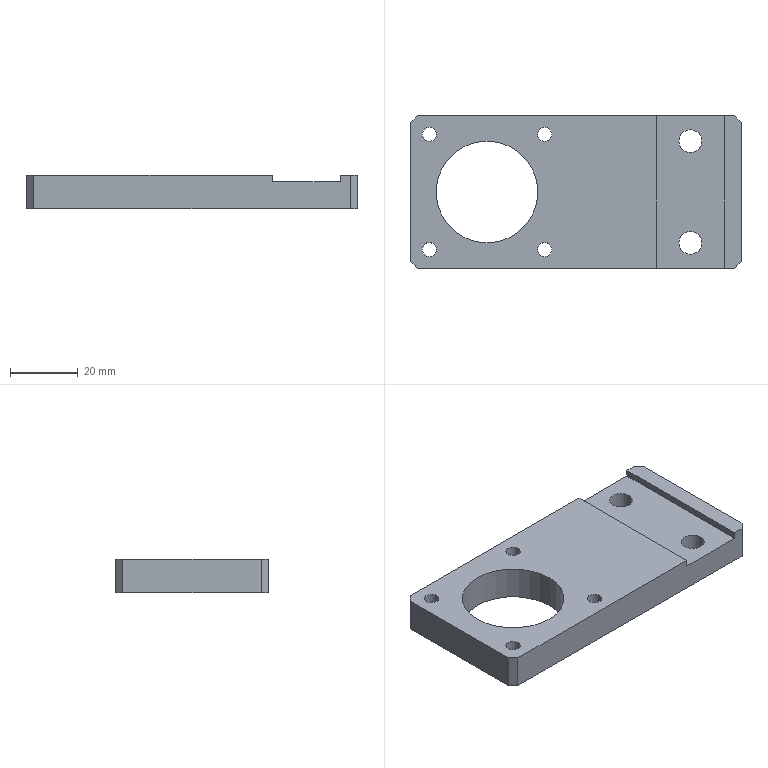Part | SolidWorks | features Chamfer 1, Extrusion 1, HoleWzd 1, ICE 1 | 1 solid | 28 faces | box 97.5 x 45 x 10 mm | volume 33791 mm3 | cylinder 14 | plane 14 | commonest cylinder face diameters 4.2 x8 6.8 x4 30 x2
STEP:
#1=CARTESIAN_POINT('',(41.6,5.5,10.));
#2=VERTEX_POINT('',#1);
#3=CARTESIAN_POINT('',(37.4,5.5,10.));
#4=VERTEX_POINT('',#3);
#5=CARTESIAN_POINT('',(39.5,5.5,10.));
#6=DIRECTION('',(0.,0.,-1.));
#7=DIRECTION('',(-1.,0.,0.));
#8=AXIS2_PLACEMENT_3D('',#5,#6,#7);
#9=CIRCLE('',#8,2.1);
#10=EDGE_CURVE('',#2,#4,#9,.T.);
#11=ORIENTED_EDGE('',*,*,#10,.F.);
#12=CARTESIAN_POINT('',(41.6,5.5,0.));
#13=VERTEX_POINT('',#12);
#14=CARTESIAN_POINT('',(41.6,5.5,0.));
#15=DIRECTION('',(0.,0.,-1.));
#16=VECTOR('',#15,1000.);
#17=LINE('',#14,#16);
#18=EDGE_CURVE('',#2,#13,#17,.T.);
#19=ORIENTED_EDGE('',*,*,#18,.T.);
#20=CARTESIAN_POINT('',(37.4,5.5,0.));
#21=VERTEX_POINT('',#20);
#22=CARTESIAN_POINT('',(39.5,5.5,0.));
#23=DIRECTION('',(0.,0.,-1.));
#24=DIRECTION('',(-1.,0.,0.));
#25=AXIS2_PLACEMENT_3D('',#22,#23,#24);
#26=CIRCLE('',#25,2.1);
#27=EDGE_CURVE('',#13,#21,#26,.T.);
#28=ORIENTED_EDGE('',*,*,#27,.T.);
#29=CARTESIAN_POINT('',(37.4,5.5,0.));
#30=DIRECTION('',(0.,0.,-1.));
#31=VECTOR('',#30,1000.);
#32=LINE('',#29,#31);
#33=EDGE_CURVE('',#4,#21,#32,.T.);
#34=ORIENTED_EDGE('',*,*,#33,.F.);
#35=EDGE_LOOP('',(#11,#19,#28,#34));
#36=FACE_OUTER_BOUND('',#35,.T.);
#37=CARTESIAN_POINT('',(39.5,5.5,0.));
#38=DIRECTION('',(0.,0.,-1.));
#39=DIRECTION('',(-1.,0.,0.));
#40=AXIS2_PLACEMENT_3D('',#37,#38,#39);
#41=CYLINDRICAL_SURFACE('',#40,2.1);
#42=ADVANCED_FACE('',(#36),#41,.F.);
#43=CARTESIAN_POINT('',(7.6,5.5,10.));
#44=VERTEX_POINT('',#43);
#45=CARTESIAN_POINT('',(3.4,5.5,10.));
#46=VERTEX_POINT('',#45);
#47=CARTESIAN_POINT('',(5.5,5.5,10.));
#48=DIRECTION('',(0.,0.,-1.));
#49=DIRECTION('',(-1.,0.,0.));
#50=AXIS2_PLACEMENT_3D('',#47,#48,#49);
#51=CIRCLE('',#50,2.1);
#52=EDGE_CURVE('',#44,#46,#51,.T.);
#53=ORIENTED_EDGE('',*,*,#52,.F.);
#54=CARTESIAN_POINT('',(7.6,5.5,0.));
#55=VERTEX_POINT('',#54);
#56=CARTESIAN_POINT('',(7.6,5.5,0.));
#57=DIRECTION('',(0.,0.,-1.));
#58=VECTOR('',#57,1000.);
#59=LINE('',#56,#58);
#60=EDGE_CURVE('',#44,#55,#59,.T.);
#61=ORIENTED_EDGE('',*,*,#60,.T.);
#62=CARTESIAN_POINT('',(3.4,5.5,0.));
#63=VERTEX_POINT('',#62);
#64=CARTESIAN_POINT('',(5.5,5.5,0.));
#65=DIRECTION('',(0.,0.,-1.));
#66=DIRECTION('',(-1.,0.,0.));
#67=AXIS2_PLACEMENT_3D('',#64,#65,#66);
#68=CIRCLE('',#67,2.1);
#69=EDGE_CURVE('',#55,#63,#68,.T.);
#70=ORIENTED_EDGE('',*,*,#69,.T.);
#71=CARTESIAN_POINT('',(3.4,5.5,0.));
#72=DIRECTION('',(0.,0.,-1.));
#73=VECTOR('',#72,1000.);
#74=LINE('',#71,#73);
#75=EDGE_CURVE('',#46,#63,#74,.T.);
#76=ORIENTED_EDGE('',*,*,#75,.F.);
#77=EDGE_LOOP('',(#53,#61,#70,#76));
#78=FACE_OUTER_BOUND('',#77,.T.);
#79=CARTESIAN_POINT('',(5.5,5.5,0.));
#80=DIRECTION('',(0.,0.,-1.));
#81=DIRECTION('',(-1.,0.,0.));
#82=AXIS2_PLACEMENT_3D('',#79,#80,#81);
#83=CYLINDRICAL_SURFACE('',#82,2.1);
#84=ADVANCED_FACE('',(#78),#83,.F.);
#85=CARTESIAN_POINT('',(7.6,39.5,10.));
#86=VERTEX_POINT('',#85);
#87=CARTESIAN_POINT('',(3.4,39.5,10.));
#88=VERTEX_POINT('',#87);
#89=CARTESIAN_POINT('',(5.5,39.5,10.));
#90=DIRECTION('',(0.,0.,-1.));
#91=DIRECTION('',(-1.,0.,0.));
#92=AXIS2_PLACEMENT_3D('',#89,#90,#91);
#93=CIRCLE('',#92,2.1);
#94=EDGE_CURVE('',#86,#88,#93,.T.);
#95=ORIENTED_EDGE('',*,*,#94,.F.);
#96=CARTESIAN_POINT('',(7.6,39.5,0.));
#97=VERTEX_POINT('',#96);
#98=CARTESIAN_POINT('',(7.6,39.5,0.));
#99=DIRECTION('',(0.,0.,-1.));
#100=VECTOR('',#99,1000.);
#101=LINE('',#98,#100);
#102=EDGE_CURVE('',#86,#97,#101,.T.);
#103=ORIENTED_EDGE('',*,*,#102,.T.);
#104=CARTESIAN_POINT('',(3.4,39.5,0.));
#105=VERTEX_POINT('',#104);
#106=CARTESIAN_POINT('',(5.5,39.5,0.));
#107=DIRECTION('',(0.,0.,-1.));
#108=DIRECTION('',(-1.,0.,0.));
#109=AXIS2_PLACEMENT_3D('',#106,#107,#108);
#110=CIRCLE('',#109,2.1);
#111=EDGE_CURVE('',#97,#105,#110,.T.);
#112=ORIENTED_EDGE('',*,*,#111,.T.);
#113=CARTESIAN_POINT('',(3.4,39.5,0.));
#114=DIRECTION('',(0.,0.,-1.));
#115=VECTOR('',#114,1000.);
#116=LINE('',#113,#115);
#117=EDGE_CURVE('',#88,#105,#116,.T.);
#118=ORIENTED_EDGE('',*,*,#117,.F.);
#119=EDGE_LOOP('',(#95,#103,#112,#118));
#120=FACE_OUTER_BOUND('',#119,.T.);
#121=CARTESIAN_POINT('',(5.5,39.5,0.));
#122=DIRECTION('',(0.,0.,-1.));
#123=DIRECTION('',(-1.,0.,0.));
#124=AXIS2_PLACEMENT_3D('',#121,#122,#123);
#125=CYLINDRICAL_SURFACE('',#124,2.1);
#126=ADVANCED_FACE('',(#120),#125,.F.);
#127=CARTESIAN_POINT('',(41.6,39.5,10.));
#128=VERTEX_POINT('',#127);
#129=CARTESIAN_POINT('',(37.4,39.5,10.));
#130=VERTEX_POINT('',#129);
#131=CARTESIAN_POINT('',(39.5,39.5,10.));
#132=DIRECTION('',(0.,0.,-1.));
#133=DIRECTION('',(-1.,0.,0.));
#134=AXIS2_PLACEMENT_3D('',#131,#132,#133);
#135=CIRCLE('',#134,2.1);
#136=EDGE_CURVE('',#128,#130,#135,.T.);
#137=ORIENTED_EDGE('',*,*,#136,.F.);
#138=CARTESIAN_POINT('',(41.6,39.5,0.));
#139=VERTEX_POINT('',#138);
#140=CARTESIAN_POINT('',(41.6,39.5,0.));
#141=DIRECTION('',(0.,0.,-1.));
#142=VECTOR('',#141,1000.);
#143=LINE('',#140,#142);
#144=EDGE_CURVE('',#128,#139,#143,.T.);
#145=ORIENTED_EDGE('',*,*,#144,.T.);
#146=CARTESIAN_POINT('',(37.4,39.5,0.));
#147=VERTEX_POINT('',#146);
#148=CARTESIAN_POINT('',(39.5,39.5,0.));
#149=DIRECTION('',(0.,0.,-1.));
#150=DIRECTION('',(-1.,0.,0.));
#151=AXIS2_PLACEMENT_3D('',#148,#149,#150);
#152=CIRCLE('',#151,2.1);
#153=EDGE_CURVE('',#139,#147,#152,.T.);
#154=ORIENTED_EDGE('',*,*,#153,.T.);
#155=CARTESIAN_POINT('',(37.4,39.5,0.));
#156=DIRECTION('',(0.,0.,-1.));
#157=VECTOR('',#156,1000.);
#158=LINE('',#155,#157);
#159=EDGE_CURVE('',#130,#147,#158,.T.);
#160=ORIENTED_EDGE('',*,*,#159,.F.);
#161=EDGE_LOOP('',(#137,#145,#154,#160));
#162=FACE_OUTER_BOUND('',#161,.T.);
#163=CARTESIAN_POINT('',(39.5,39.5,0.));
#164=DIRECTION('',(0.,0.,-1.));
#165=DIRECTION('',(-1.,0.,0.));
#166=AXIS2_PLACEMENT_3D('',#163,#164,#165);
#167=CYLINDRICAL_SURFACE('',#166,2.1);
#168=ADVANCED_FACE('',(#162),#167,.F.);
#169=CARTESIAN_POINT('',(79.1,7.5,8.));
#170=VERTEX_POINT('',#169);
#171=CARTESIAN_POINT('',(85.9,7.5,8.));
#172=VERTEX_POINT('',#171);
#173=CARTESIAN_POINT('',(82.5,7.5,8.));
#174=DIRECTION('',(0.,0.,1.));
#175=DIRECTION('',(-1.,0.,0.));
#176=AXIS2_PLACEMENT_3D('',#173,#174,#175);
#177=CIRCLE('',#176,3.4);
#178=EDGE_CURVE('',#170,#172,#177,.T.);
#179=ORIENTED_EDGE('',*,*,#178,.T.);
#180=CARTESIAN_POINT('',(85.9,7.5,0.));
#181=VERTEX_POINT('',#180);
#182=CARTESIAN_POINT('',(85.9,7.5,10.));
#183=DIRECTION('',(0.,0.,-1.));
#184=VECTOR('',#183,1000.);
#185=LINE('',#182,#184);
#186=EDGE_CURVE('',#172,#181,#185,.T.);
#187=ORIENTED_EDGE('',*,*,#186,.T.);
#188=CARTESIAN_POINT('',(79.1,7.5,0.));
#189=VERTEX_POINT('',#188);
#190=CARTESIAN_POINT('',(82.5,7.5,0.));
#191=DIRECTION('',(0.,0.,1.));
#192=DIRECTION('',(1.,0.,0.));
#193=AXIS2_PLACEMENT_3D('',#190,#191,#192);
#194=CIRCLE('',#193,3.4);
#195=EDGE_CURVE('',#189,#181,#194,.T.);
#196=ORIENTED_EDGE('',*,*,#195,.F.);
#197=CARTESIAN_POINT('',(79.1,7.5,10.));
#198=DIRECTION('',(0.,0.,-1.));
#199=VECTOR('',#198,1000.);
#200=LINE('',#197,#199);
#201=EDGE_CURVE('',#170,#189,#200,.T.);
#202=ORIENTED_EDGE('',*,*,#201,.F.);
#203=EDGE_LOOP('',(#179,#187,#196,#202));
#204=FACE_OUTER_BOUND('',#203,.T.);
#205=CARTESIAN_POINT('',(82.5,7.5,10.));
#206=DIRECTION('',(0.,0.,-1.));
#207=DIRECTION('',(-1.,0.,0.));
#208=AXIS2_PLACEMENT_3D('',#205,#206,#207);
#209=CYLINDRICAL_SURFACE('',#208,3.4);
#210=ADVANCED_FACE('',(#204),#209,.F.);
#211=CARTESIAN_POINT('',(79.1,37.5,8.));
#212=VERTEX_POINT('',#211);
#213=CARTESIAN_POINT('',(85.9,37.5,8.));
#214=VERTEX_POINT('',#213);
#215=CARTESIAN_POINT('',(82.5,37.5,8.));
#216=DIRECTION('',(0.,0.,1.));
#217=DIRECTION('',(-1.,0.,0.));
#218=AXIS2_PLACEMENT_3D('',#215,#216,#217);
#219=CIRCLE('',#218,3.4);
#220=EDGE_CURVE('',#212,#214,#219,.T.);
#221=ORIENTED_EDGE('',*,*,#220,.T.);
#222=CARTESIAN_POINT('',(85.9,37.5,0.));
#223=VERTEX_POINT('',#222);
#224=CARTESIAN_POINT('',(85.9,37.5,10.));
#225=DIRECTION('',(0.,0.,-1.));
#226=VECTOR('',#225,1000.);
#227=LINE('',#224,#226);
#228=EDGE_CURVE('',#214,#223,#227,.T.);
#229=ORIENTED_EDGE('',*,*,#228,.T.);
#230=CARTESIAN_POINT('',(79.1,37.5,0.));
#231=VERTEX_POINT('',#230);
#232=CARTESIAN_POINT('',(82.5,37.5,0.));
#233=DIRECTION('',(0.,0.,1.));
#234=DIRECTION('',(1.,0.,0.));
#235=AXIS2_PLACEMENT_3D('',#232,#233,#234);
#236=CIRCLE('',#235,3.4);
#237=EDGE_CURVE('',#231,#223,#236,.T.);
#238=ORIENTED_EDGE('',*,*,#237,.F.);
#239=CARTESIAN_POINT('',(79.1,37.5,10.));
#240=DIRECTION('',(0.,0.,-1.));
#241=VECTOR('',#240,1000.);
#242=LINE('',#239,#241);
#243=EDGE_CURVE('',#212,#231,#242,.T.);
#244=ORIENTED_EDGE('',*,*,#243,.F.);
#245=EDGE_LOOP('',(#221,#229,#238,#244));
#246=FACE_OUTER_BOUND('',#245,.T.);
#247=CARTESIAN_POINT('',(82.5,37.5,10.));
#248=DIRECTION('',(0.,0.,-1.));
#249=DIRECTION('',(-1.,0.,0.));
#250=AXIS2_PLACEMENT_3D('',#247,#248,#249);
#251=CYLINDRICAL_SURFACE('',#250,3.4);
#252=ADVANCED_FACE('',(#246),#251,.F.);
#253=CARTESIAN_POINT('',(7.5,22.5,10.));
#254=VERTEX_POINT('',#253);
#255=CARTESIAN_POINT('',(37.5,22.5,10.));
#256=VERTEX_POINT('',#255);
#257=CARTESIAN_POINT('',(22.5,22.5,10.));
#258=DIRECTION('',(0.,0.,1.));
#259=DIRECTION('',(1.,0.,0.));
#260=AXIS2_PLACEMENT_3D('',#257,#258,#259);
#261=CIRCLE('',#260,15.);
#262=EDGE_CURVE('',#254,#256,#261,.T.);
#263=ORIENTED_EDGE('',*,*,#262,.T.);
#264=CARTESIAN_POINT('',(37.5,22.5,0.));
#265=VERTEX_POINT('',#264);
#266=CARTESIAN_POINT('',(37.5,22.5,10.));
#267=DIRECTION('',(0.,0.,-1.));
#268=VECTOR('',#267,1000.);
#269=LINE('',#266,#268);
#270=EDGE_CURVE('',#256,#265,#269,.T.);
#271=ORIENTED_EDGE('',*,*,#270,.T.);
#272=CARTESIAN_POINT('',(7.5,22.5,0.));
#273=VERTEX_POINT('',#272);
#274=CARTESIAN_POINT('',(22.5,22.5,0.));
#275=DIRECTION('',(0.,0.,1.));
#276=DIRECTION('',(1.,0.,0.));
#277=AXIS2_PLACEMENT_3D('',#274,#275,#276);
#278=CIRCLE('',#277,15.);
#279=EDGE_CURVE('',#273,#265,#278,.T.);
#280=ORIENTED_EDGE('',*,*,#279,.F.);
#281=CARTESIAN_POINT('',(7.5,22.5,10.));
#282=DIRECTION('',(0.,0.,-1.));
#283=VECTOR('',#282,1000.);
#284=LINE('',#281,#283);
#285=EDGE_CURVE('',#254,#273,#284,.T.);
#286=ORIENTED_EDGE('',*,*,#285,.F.);
#287=EDGE_LOOP('',(#263,#271,#280,#286));
#288=FACE_OUTER_BOUND('',#287,.T.);
#289=CARTESIAN_POINT('',(22.5,22.5,10.));
#290=DIRECTION('',(0.,0.,-1.));
#291=DIRECTION('',(-1.,0.,0.));
#292=AXIS2_PLACEMENT_3D('',#289,#290,#291);
#293=CYLINDRICAL_SURFACE('',#292,15.);
#294=ADVANCED_FACE('',(#288),#293,.F.);
#295=CARTESIAN_POINT('',(39.5,5.5,10.));
#296=DIRECTION('',(0.,0.,-1.));
#297=DIRECTION('',(-1.,0.,0.));
#298=AXIS2_PLACEMENT_3D('',#295,#296,#297);
#299=CIRCLE('',#298,2.1);
#300=EDGE_CURVE('',#4,#2,#299,.T.);
#301=ORIENTED_EDGE('',*,*,#300,.T.);
#302=ORIENTED_EDGE('',*,*,#10,.T.);
#303=EDGE_LOOP('',(#301,#302));
#304=FACE_BOUND('',#303,.T.);
#305=CARTESIAN_POINT('',(5.5,5.5,10.));
#306=DIRECTION('',(0.,0.,-1.));
#307=DIRECTION('',(-1.,0.,0.));
#308=AXIS2_PLACEMENT_3D('',#305,#306,#307);
#309=CIRCLE('',#308,2.1);
#310=EDGE_CURVE('',#46,#44,#309,.T.);
#311=ORIENTED_EDGE('',*,*,#310,.T.);
#312=ORIENTED_EDGE('',*,*,#52,.T.);
#313=EDGE_LOOP('',(#311,#312));
#314=FACE_BOUND('',#313,.T.);
#315=CARTESIAN_POINT('',(5.5,39.5,10.));
#316=DIRECTION('',(0.,0.,-1.));
#317=DIRECTION('',(-1.,0.,0.));
#318=AXIS2_PLACEMENT_3D('',#315,#316,#317);
#319=CIRCLE('',#318,2.1);
#320=EDGE_CURVE('',#88,#86,#319,.T.);
#321=ORIENTED_EDGE('',*,*,#320,.T.);
#322=ORIENTED_EDGE('',*,*,#94,.T.);
#323=EDGE_LOOP('',(#321,#322));
#324=FACE_BOUND('',#323,.T.);
#325=CARTESIAN_POINT('',(39.5,39.5,10.));
#326=DIRECTION('',(0.,0.,-1.));
#327=DIRECTION('',(-1.,0.,0.));
#328=AXIS2_PLACEMENT_3D('',#325,#326,#327);
#329=CIRCLE('',#328,2.1);
#330=EDGE_CURVE('',#130,#128,#329,.T.);
#331=ORIENTED_EDGE('',*,*,#330,.T.);
#332=ORIENTED_EDGE('',*,*,#136,.T.);
#333=EDGE_LOOP('',(#331,#332));
#334=FACE_BOUND('',#333,.T.);
#335=ORIENTED_EDGE('',*,*,#262,.F.);
#336=CARTESIAN_POINT('',(22.5,22.5,10.));
#337=DIRECTION('',(0.,0.,1.));
#338=DIRECTION('',(1.,0.,0.));
#339=AXIS2_PLACEMENT_3D('',#336,#337,#338);
#340=CIRCLE('',#339,15.);
#341=EDGE_CURVE('',#256,#254,#340,.T.);
#342=ORIENTED_EDGE('',*,*,#341,.F.);
#343=EDGE_LOOP('',(#335,#342));
#344=FACE_BOUND('',#343,.T.);
#345=CARTESIAN_POINT('',(0.,43.,10.));
#346=VERTEX_POINT('',#345);
#347=CARTESIAN_POINT('',(0.,2.,10.));
#348=VERTEX_POINT('',#347);
#349=CARTESIAN_POINT('',(0.,0.,10.));
#350=DIRECTION('',(0.,-1.,0.));
#351=VECTOR('',#350,1000.);
#352=LINE('',#349,#351);
#353=EDGE_CURVE('',#346,#348,#352,.T.);
#354=ORIENTED_EDGE('',*,*,#353,.T.);
#355=CARTESIAN_POINT('',(2.,0.,10.));
#356=VERTEX_POINT('',#355);
#357=CARTESIAN_POINT('',(2.,0.,10.));
#358=DIRECTION('',(0.7071,-0.7071,0.));
#359=VECTOR('',#358,1000.);
#360=LINE('',#357,#359);
#361=EDGE_CURVE('',#348,#356,#360,.T.);
#362=ORIENTED_EDGE('',*,*,#361,.T.);
#363=CARTESIAN_POINT('',(72.5,0.,10.));
#364=VERTEX_POINT('',#363);
#365=CARTESIAN_POINT('',(0.,0.,10.));
#366=DIRECTION('',(1.,0.,0.));
#367=VECTOR('',#366,1000.);
#368=LINE('',#365,#367);
#369=EDGE_CURVE('',#356,#364,#368,.T.);
#370=ORIENTED_EDGE('',*,*,#369,.T.);
#371=CARTESIAN_POINT('',(72.5,45.,10.));
#372=VERTEX_POINT('',#371);
#373=CARTESIAN_POINT('',(72.5,-0.001,10.));
#374=DIRECTION('',(0.,1.,0.));
#375=VECTOR('',#374,1000.);
#376=LINE('',#373,#375);
#377=EDGE_CURVE('',#364,#372,#376,.T.);
#378=ORIENTED_EDGE('',*,*,#377,.T.);
#379=CARTESIAN_POINT('',(2.,45.,10.));
#380=VERTEX_POINT('',#379);
#381=CARTESIAN_POINT('',(0.,45.,10.));
#382=DIRECTION('',(-1.,0.,0.));
#383=VECTOR('',#382,1000.);
#384=LINE('',#381,#383);
#385=EDGE_CURVE('',#372,#380,#384,.T.);
#386=ORIENTED_EDGE('',*,*,#385,.T.);
#387=CARTESIAN_POINT('',(0.,43.,10.));
#388=DIRECTION('',(-0.7071,-0.7071,0.));
#389=VECTOR('',#388,1000.);
#390=LINE('',#387,#389);
#391=EDGE_CURVE('',#380,#346,#390,.T.);
#392=ORIENTED_EDGE('',*,*,#391,.T.);
#393=EDGE_LOOP('',(#354,#362,#370,#378,#386,#392));
#394=FACE_OUTER_BOUND('',#393,.T.);
#395=CARTESIAN_POINT('',(0.,45.,10.));
#396=DIRECTION('',(0.,0.,-1.));
#397=DIRECTION('',(-1.,0.,0.));
#398=AXIS2_PLACEMENT_3D('',#395,#396,#397);
#399=PLANE('',#398);
#400=ADVANCED_FACE('',(#304,#314,#324,#334,#344,#394),#399,.F.);
#401=CARTESIAN_POINT('',(92.5,0.,10.));
#402=VERTEX_POINT('',#401);
#403=CARTESIAN_POINT('',(95.5,0.,10.));
#404=VERTEX_POINT('',#403);
#405=CARTESIAN_POINT('',(0.,0.,10.));
#406=DIRECTION('',(1.,0.,0.));
#407=VECTOR('',#406,1000.);
#408=LINE('',#405,#407);
#409=EDGE_CURVE('',#402,#404,#408,.T.);
#410=ORIENTED_EDGE('',*,*,#409,.T.);
#411=CARTESIAN_POINT('',(97.5,2.,10.));
#412=VERTEX_POINT('',#411);
#413=CARTESIAN_POINT('',(97.5,2.,10.));
#414=DIRECTION('',(0.7071,0.7071,0.));
#415=VECTOR('',#414,1000.);
#416=LINE('',#413,#415);
#417=EDGE_CURVE('',#404,#412,#416,.T.);
#418=ORIENTED_EDGE('',*,*,#417,.T.);
#419=CARTESIAN_POINT('',(97.5,43.,10.));
#420=VERTEX_POINT('',#419);
#421=CARTESIAN_POINT('',(97.5,0.,10.));
#422=DIRECTION('',(0.,1.,0.));
#423=VECTOR('',#422,1000.);
#424=LINE('',#421,#423);
#425=EDGE_CURVE('',#412,#420,#424,.T.);
#426=ORIENTED_EDGE('',*,*,#425,.T.);
#427=CARTESIAN_POINT('',(95.5,45.,10.));
#428=VERTEX_POINT('',#427);
#429=CARTESIAN_POINT('',(95.5,45.,10.));
#430=DIRECTION('',(-0.7071,0.7071,0.));
#431=VECTOR('',#430,1000.);
#432=LINE('',#429,#431);
#433=EDGE_CURVE('',#420,#428,#432,.T.);
#434=ORIENTED_EDGE('',*,*,#433,.T.);
#435=CARTESIAN_POINT('',(92.5,45.,10.));
#436=VERTEX_POINT('',#435);
#437=CARTESIAN_POINT('',(0.,45.,10.));
#438=DIRECTION('',(-1.,0.,0.));
#439=VECTOR('',#438,1000.);
#440=LINE('',#437,#439);
#441=EDGE_CURVE('',#428,#436,#440,.T.);
#442=ORIENTED_EDGE('',*,*,#441,.T.);
#443=CARTESIAN_POINT('',(92.5,-0.001,10.));
#444=DIRECTION('',(0.,1.,0.));
#445=VECTOR('',#444,1000.);
#446=LINE('',#443,#445);
#447=EDGE_CURVE('',#402,#436,#446,.T.);
#448=ORIENTED_EDGE('',*,*,#447,.F.);
#449=EDGE_LOOP('',(#410,#418,#426,#434,#442,#448));
#450=FACE_OUTER_BOUND('',#449,.T.);
#451=CARTESIAN_POINT('',(0.,45.,10.));
#452=DIRECTION('',(0.,0.,-1.));
#453=DIRECTION('',(-1.,0.,0.));
#454=AXIS2_PLACEMENT_3D('',#451,#452,#453);
#455=PLANE('',#454);
#456=ADVANCED_FACE('',(#450),#455,.F.);
#457=CARTESIAN_POINT('',(39.5,5.5,0.));
#458=DIRECTION('',(0.,0.,-1.));
#459=DIRECTION('',(-1.,0.,0.));
#460=AXIS2_PLACEMENT_3D('',#457,#458,#459);
#461=CIRCLE('',#460,2.1);
#462=EDGE_CURVE('',#21,#13,#461,.T.);
#463=ORIENTED_EDGE('',*,*,#462,.F.);
#464=ORIENTED_EDGE('',*,*,#27,.F.);
#465=EDGE_LOOP('',(#463,#464));
#466=FACE_BOUND('',#465,.T.);
#467=CARTESIAN_POINT('',(5.5,5.5,0.));
#468=DIRECTION('',(0.,0.,-1.));
#469=DIRECTION('',(-1.,0.,0.));
#470=AXIS2_PLACEMENT_3D('',#467,#468,#469);
#471=CIRCLE('',#470,2.1);
#472=EDGE_CURVE('',#63,#55,#471,.T.);
#473=ORIENTED_EDGE('',*,*,#472,.F.);
#474=ORIENTED_EDGE('',*,*,#69,.F.);
#475=EDGE_LOOP('',(#473,#474));
#476=FACE_BOUND('',#475,.T.);
#477=CARTESIAN_POINT('',(5.5,39.5,0.));
#478=DIRECTION('',(0.,0.,-1.));
#479=DIRECTION('',(-1.,0.,0.));
#480=AXIS2_PLACEMENT_3D('',#477,#478,#479);
#481=CIRCLE('',#480,2.1);
#482=EDGE_CURVE('',#105,#97,#481,.T.);
#483=ORIENTED_EDGE('',*,*,#482,.F.);
#484=ORIENTED_EDGE('',*,*,#111,.F.);
#485=EDGE_LOOP('',(#483,#484));
#486=FACE_BOUND('',#485,.T.);
#487=CARTESIAN_POINT('',(39.5,39.5,0.));
#488=DIRECTION('',(0.,0.,-1.));
#489=DIRECTION('',(-1.,0.,0.));
#490=AXIS2_PLACEMENT_3D('',#487,#488,#489);
#491=CIRCLE('',#490,2.1);
#492=EDGE_CURVE('',#147,#139,#491,.T.);
#493=ORIENTED_EDGE('',*,*,#492,.F.);
#494=ORIENTED_EDGE('',*,*,#153,.F.);
#495=EDGE_LOOP('',(#493,#494));
#496=FACE_BOUND('',#495,.T.);
#497=ORIENTED_EDGE('',*,*,#237,.T.);
#498=CARTESIAN_POINT('',(82.5,37.5,0.));
#499=DIRECTION('',(0.,0.,1.));
#500=DIRECTION('',(1.,0.,0.));
#501=AXIS2_PLACEMENT_3D('',#498,#499,#500);
#502=CIRCLE('',#501,3.4);
#503=EDGE_CURVE('',#223,#231,#502,.T.);
#504=ORIENTED_EDGE('',*,*,#503,.T.);
#505=EDGE_LOOP('',(#497,#504));
#506=FACE_BOUND('',#505,.T.);
#507=CARTESIAN_POINT('',(97.5,2.,0.));
#508=VERTEX_POINT('',#507);
#509=CARTESIAN_POINT('',(97.5,43.,0.));
#510=VERTEX_POINT('',#509);
#511=CARTESIAN_POINT('',(97.5,0.,0.));
#512=DIRECTION('',(0.,1.,0.));
#513=VECTOR('',#512,1000.);
#514=LINE('',#511,#513);
#515=EDGE_CURVE('',#508,#510,#514,.T.);
#516=ORIENTED_EDGE('',*,*,#515,.F.);
#517=CARTESIAN_POINT('',(95.5,0.,0.));
#518=VERTEX_POINT('',#517);
#519=CARTESIAN_POINT('',(70.25,-25.25,0.));
#520=DIRECTION('',(-0.7071,-0.7071,0.));
#521=VECTOR('',#520,1000.);
#522=LINE('',#519,#521);
#523=EDGE_CURVE('',#508,#518,#522,.T.);
#524=ORIENTED_EDGE('',*,*,#523,.T.);
#525=CARTESIAN_POINT('',(2.,0.,0.));
#526=VERTEX_POINT('',#525);
#527=CARTESIAN_POINT('',(0.,0.,0.));
#528=DIRECTION('',(1.,0.,0.));
#529=VECTOR('',#528,1000.);
#530=LINE('',#527,#529);
#531=EDGE_CURVE('',#526,#518,#530,.T.);
#532=ORIENTED_EDGE('',*,*,#531,.F.);
#533=CARTESIAN_POINT('',(0.,2.,0.));
#534=VERTEX_POINT('',#533);
#535=CARTESIAN_POINT('',(-21.5,23.5,0.));
#536=DIRECTION('',(-0.7071,0.7071,0.));
#537=VECTOR('',#536,1000.);
#538=LINE('',#535,#537);
#539=EDGE_CURVE('',#526,#534,#538,.T.);
#540=ORIENTED_EDGE('',*,*,#539,.T.);
#541=CARTESIAN_POINT('',(0.,43.,0.));
#542=VERTEX_POINT('',#541);
#543=CARTESIAN_POINT('',(0.,0.,0.));
#544=DIRECTION('',(0.,-1.,0.));
#545=VECTOR('',#544,1000.);
#546=LINE('',#543,#545);
#547=EDGE_CURVE('',#542,#534,#546,.T.);
#548=ORIENTED_EDGE('',*,*,#547,.F.);
#549=CARTESIAN_POINT('',(2.,45.,0.));
#550=VERTEX_POINT('',#549);
#551=CARTESIAN_POINT('',(1.,44.,0.));
#552=DIRECTION('',(0.7071,0.7071,0.));
#553=VECTOR('',#552,1000.);
#554=LINE('',#551,#553);
#555=EDGE_CURVE('',#542,#550,#554,.T.);
#556=ORIENTED_EDGE('',*,*,#555,.T.);
#557=CARTESIAN_POINT('',(95.5,45.,0.));
#558=VERTEX_POINT('',#557);
#559=CARTESIAN_POINT('',(0.,45.,0.));
#560=DIRECTION('',(-1.,0.,0.));
#561=VECTOR('',#560,1000.);
#562=LINE('',#559,#561);
#563=EDGE_CURVE('',#558,#550,#562,.T.);
#564=ORIENTED_EDGE('',*,*,#563,.F.);
#565=CARTESIAN_POINT('',(47.75,92.75,0.));
#566=DIRECTION('',(0.7071,-0.7071,0.));
#567=VECTOR('',#566,1000.);
#568=LINE('',#565,#567);
#569=EDGE_CURVE('',#558,#510,#568,.T.);
#570=ORIENTED_EDGE('',*,*,#569,.T.);
#571=EDGE_LOOP('',(#516,#524,#532,#540,#548,#556,#564,#570));
#572=FACE_OUTER_BOUND('',#571,.T.);
#573=ORIENTED_EDGE('',*,*,#279,.T.);
#574=CARTESIAN_POINT('',(22.5,22.5,0.));
#575=DIRECTION('',(0.,0.,1.));
#576=DIRECTION('',(1.,0.,0.));
#577=AXIS2_PLACEMENT_3D('',#574,#575,#576);
#578=CIRCLE('',#577,15.);
#579=EDGE_CURVE('',#265,#273,#578,.T.);
#580=ORIENTED_EDGE('',*,*,#579,.T.);
#581=EDGE_LOOP('',(#573,#580));
#582=FACE_BOUND('',#581,.T.);
#583=ORIENTED_EDGE('',*,*,#195,.T.);
#584=CARTESIAN_POINT('',(82.5,7.5,0.));
#585=DIRECTION('',(0.,0.,1.));
#586=DIRECTION('',(1.,0.,0.));
#587=AXIS2_PLACEMENT_3D('',#584,#585,#586);
#588=CIRCLE('',#587,3.4);
#589=EDGE_CURVE('',#181,#189,#588,.T.);
#590=ORIENTED_EDGE('',*,*,#589,.T.);
#591=EDGE_LOOP('',(#583,#590));
#592=FACE_BOUND('',#591,.T.);
#593=CARTESIAN_POINT('',(0.,45.,0.));
#594=DIRECTION('',(0.,0.,-1.));
#595=DIRECTION('',(-1.,0.,0.));
#596=AXIS2_PLACEMENT_3D('',#593,#594,#595);
#597=PLANE('',#596);
#598=ADVANCED_FACE('',(#466,#476,#486,#496,#506,#572,#582,#592),#597,.T.);
#599=ORIENTED_EDGE('',*,*,#547,.T.);
#600=CARTESIAN_POINT('',(0.,2.,10.));
#601=DIRECTION('',(0.,0.,1.));
#602=VECTOR('',#601,1000.);
#603=LINE('',#600,#602);
#604=EDGE_CURVE('',#534,#348,#603,.T.);
#605=ORIENTED_EDGE('',*,*,#604,.T.);
#606=ORIENTED_EDGE('',*,*,#353,.F.);
#607=CARTESIAN_POINT('',(0.,43.,10.));
#608=DIRECTION('',(0.,0.,-1.));
#609=VECTOR('',#608,1000.);
#610=LINE('',#607,#609);
#611=EDGE_CURVE('',#346,#542,#610,.T.);
#612=ORIENTED_EDGE('',*,*,#611,.T.);
#613=EDGE_LOOP('',(#599,#605,#606,#612));
#614=FACE_OUTER_BOUND('',#613,.T.);
#615=CARTESIAN_POINT('',(0.,0.,10.));
#616=DIRECTION('',(1.,0.,0.));
#617=DIRECTION('',(0.,0.,-1.));
#618=AXIS2_PLACEMENT_3D('',#615,#616,#617);
#619=PLANE('',#618);
#620=ADVANCED_FACE('',(#614),#619,.F.);
#621=ORIENTED_EDGE('',*,*,#531,.T.);
#622=CARTESIAN_POINT('',(95.5,0.,10.));
#623=DIRECTION('',(0.,0.,1.));
#624=VECTOR('',#623,1000.);
#625=LINE('',#622,#624);
#626=EDGE_CURVE('',#518,#404,#625,.T.);
#627=ORIENTED_EDGE('',*,*,#626,.T.);
#628=ORIENTED_EDGE('',*,*,#409,.F.);
#629=CARTESIAN_POINT('',(92.5,0.,8.));
#630=VERTEX_POINT('',#629);
#631=CARTESIAN_POINT('',(92.5,0.,10.));
#632=DIRECTION('',(0.,0.,1.));
#633=VECTOR('',#632,1000.);
#634=LINE('',#631,#633);
#635=EDGE_CURVE('',#630,#402,#634,.T.);
#636=ORIENTED_EDGE('',*,*,#635,.F.);
#637=CARTESIAN_POINT('',(72.5,0.,8.));
#638=VERTEX_POINT('',#637);
#639=CARTESIAN_POINT('',(72.5,0.,8.));
#640=DIRECTION('',(1.,0.,0.));
#641=VECTOR('',#640,1000.);
#642=LINE('',#639,#641);
#643=EDGE_CURVE('',#638,#630,#642,.T.);
#644=ORIENTED_EDGE('',*,*,#643,.F.);
#645=CARTESIAN_POINT('',(72.5,0.,10.));
#646=DIRECTION('',(0.,0.,-1.));
#647=VECTOR('',#646,1000.);
#648=LINE('',#645,#647);
#649=EDGE_CURVE('',#364,#638,#648,.T.);
#650=ORIENTED_EDGE('',*,*,#649,.F.);
#651=ORIENTED_EDGE('',*,*,#369,.F.);
#652=CARTESIAN_POINT('',(2.,0.,10.));
#653=DIRECTION('',(0.,0.,-1.));
#654=VECTOR('',#653,1000.);
#655=LINE('',#652,#654);
#656=EDGE_CURVE('',#356,#526,#655,.T.);
#657=ORIENTED_EDGE('',*,*,#656,.T.);
#658=EDGE_LOOP('',(#621,#627,#628,#636,#644,#650,#651,#657));
#659=FACE_OUTER_BOUND('',#658,.T.);
#660=CARTESIAN_POINT('',(0.,0.,10.));
#661=DIRECTION('',(0.,1.,0.));
#662=DIRECTION('',(0.,0.,1.));
#663=AXIS2_PLACEMENT_3D('',#660,#661,#662);
#664=PLANE('',#663);
#665=ADVANCED_FACE('',(#659),#664,.F.);
#666=ORIENTED_EDGE('',*,*,#425,.F.);
#667=CARTESIAN_POINT('',(97.5,2.,10.));
#668=DIRECTION('',(0.,0.,-1.));
#669=VECTOR('',#668,1000.);
#670=LINE('',#667,#669);
#671=EDGE_CURVE('',#412,#508,#670,.T.);
#672=ORIENTED_EDGE('',*,*,#671,.T.);
#673=ORIENTED_EDGE('',*,*,#515,.T.);
#674=CARTESIAN_POINT('',(97.5,43.,10.));
#675=DIRECTION('',(0.,0.,1.));
#676=VECTOR('',#675,1000.);
#677=LINE('',#674,#676);
#678=EDGE_CURVE('',#510,#420,#677,.T.);
#679=ORIENTED_EDGE('',*,*,#678,.T.);
#680=EDGE_LOOP('',(#666,#672,#673,#679));
#681=FACE_OUTER_BOUND('',#680,.T.);
#682=CARTESIAN_POINT('',(97.5,0.,10.));
#683=DIRECTION('',(-1.,0.,0.));
#684=DIRECTION('',(0.,0.,1.));
#685=AXIS2_PLACEMENT_3D('',#682,#683,#684);
#686=PLANE('',#685);
#687=ADVANCED_FACE('',(#681),#686,.F.);
#688=ORIENTED_EDGE('',*,*,#441,.F.);
#689=CARTESIAN_POINT('',(95.5,45.,10.));
#690=DIRECTION('',(0.,0.,-1.));
#691=VECTOR('',#690,1000.);
#692=LINE('',#689,#691);
#693=EDGE_CURVE('',#428,#558,#692,.T.);
#694=ORIENTED_EDGE('',*,*,#693,.T.);
#695=ORIENTED_EDGE('',*,*,#563,.T.);
#696=CARTESIAN_POINT('',(2.,45.,10.));
#697=DIRECTION('',(0.,0.,1.));
#698=VECTOR('',#697,1000.);
#699=LINE('',#696,#698);
#700=EDGE_CURVE('',#550,#380,#699,.T.);
#701=ORIENTED_EDGE('',*,*,#700,.T.);
#702=ORIENTED_EDGE('',*,*,#385,.F.);
#703=CARTESIAN_POINT('',(72.5,45.,8.));
#704=VERTEX_POINT('',#703);
#705=CARTESIAN_POINT('',(72.5,45.,10.));
#706=DIRECTION('',(0.,0.,1.));
#707=VECTOR('',#706,1000.);
#708=LINE('',#705,#707);
#709=EDGE_CURVE('',#704,#372,#708,.T.);
#710=ORIENTED_EDGE('',*,*,#709,.F.);
#711=CARTESIAN_POINT('',(92.5,45.,8.));
#712=VERTEX_POINT('',#711);
#713=CARTESIAN_POINT('',(72.5,45.,8.));
#714=DIRECTION('',(-1.,0.,0.));
#715=VECTOR('',#714,1000.);
#716=LINE('',#713,#715);
#717=EDGE_CURVE('',#712,#704,#716,.T.);
#718=ORIENTED_EDGE('',*,*,#717,.F.);
#719=CARTESIAN_POINT('',(92.5,45.,10.));
#720=DIRECTION('',(0.,0.,-1.));
#721=VECTOR('',#720,1000.);
#722=LINE('',#719,#721);
#723=EDGE_CURVE('',#436,#712,#722,.T.);
#724=ORIENTED_EDGE('',*,*,#723,.F.);
#725=EDGE_LOOP('',(#688,#694,#695,#701,#702,#710,#718,#724));
#726=FACE_OUTER_BOUND('',#725,.T.);
#727=CARTESIAN_POINT('',(0.,45.,10.));
#728=DIRECTION('',(0.,-1.,0.));
#729=DIRECTION('',(0.,0.,-1.));
#730=AXIS2_PLACEMENT_3D('',#727,#728,#729);
#731=PLANE('',#730);
#732=ADVANCED_FACE('',(#726),#731,.F.);
#733=ORIENTED_EDGE('',*,*,#270,.F.);
#734=ORIENTED_EDGE('',*,*,#341,.T.);
#735=ORIENTED_EDGE('',*,*,#285,.T.);
#736=ORIENTED_EDGE('',*,*,#579,.F.);
#737=EDGE_LOOP('',(#733,#734,#735,#736));
#738=FACE_OUTER_BOUND('',#737,.T.);
#739=CARTESIAN_POINT('',(22.5,22.5,10.));
#740=DIRECTION('',(0.,0.,-1.));
#741=DIRECTION('',(-1.,0.,0.));
#742=AXIS2_PLACEMENT_3D('',#739,#740,#741);
#743=CYLINDRICAL_SURFACE('',#742,15.);
#744=ADVANCED_FACE('',(#738),#743,.F.);
#745=ORIENTED_EDGE('',*,*,#228,.F.);
#746=CARTESIAN_POINT('',(82.5,37.5,8.));
#747=DIRECTION('',(0.,0.,1.));
#748=DIRECTION('',(-1.,0.,0.));
#749=AXIS2_PLACEMENT_3D('',#746,#747,#748);
#750=CIRCLE('',#749,3.4);
#751=EDGE_CURVE('',#214,#212,#750,.T.);
#752=ORIENTED_EDGE('',*,*,#751,.T.);
#753=ORIENTED_EDGE('',*,*,#243,.T.);
#754=ORIENTED_EDGE('',*,*,#503,.F.);
#755=EDGE_LOOP('',(#745,#752,#753,#754));
#756=FACE_OUTER_BOUND('',#755,.T.);
#757=CARTESIAN_POINT('',(82.5,37.5,10.));
#758=DIRECTION('',(0.,0.,-1.));
#759=DIRECTION('',(-1.,0.,0.));
#760=AXIS2_PLACEMENT_3D('',#757,#758,#759);
#761=CYLINDRICAL_SURFACE('',#760,3.4);
#762=ADVANCED_FACE('',(#756),#761,.F.);
#763=ORIENTED_EDGE('',*,*,#186,.F.);
#764=CARTESIAN_POINT('',(82.5,7.5,8.));
#765=DIRECTION('',(0.,0.,1.));
#766=DIRECTION('',(-1.,0.,0.));
#767=AXIS2_PLACEMENT_3D('',#764,#765,#766);
#768=CIRCLE('',#767,3.4);
#769=EDGE_CURVE('',#172,#170,#768,.T.);
#770=ORIENTED_EDGE('',*,*,#769,.T.);
#771=ORIENTED_EDGE('',*,*,#201,.T.);
#772=ORIENTED_EDGE('',*,*,#589,.F.);
#773=EDGE_LOOP('',(#763,#770,#771,#772));
#774=FACE_OUTER_BOUND('',#773,.T.);
#775=CARTESIAN_POINT('',(82.5,7.5,10.));
#776=DIRECTION('',(0.,0.,-1.));
#777=DIRECTION('',(-1.,0.,0.));
#778=AXIS2_PLACEMENT_3D('',#775,#776,#777);
#779=CYLINDRICAL_SURFACE('',#778,3.4);
#780=ADVANCED_FACE('',(#774),#779,.F.);
#781=ORIENTED_EDGE('',*,*,#649,.T.);
#782=CARTESIAN_POINT('',(72.5,-0.001,8.));
#783=DIRECTION('',(0.,1.,0.));
#784=VECTOR('',#783,1000.);
#785=LINE('',#782,#784);
#786=EDGE_CURVE('',#638,#704,#785,.T.);
#787=ORIENTED_EDGE('',*,*,#786,.T.);
#788=ORIENTED_EDGE('',*,*,#709,.T.);
#789=ORIENTED_EDGE('',*,*,#377,.F.);
#790=EDGE_LOOP('',(#781,#787,#788,#789));
#791=FACE_OUTER_BOUND('',#790,.T.);
#792=CARTESIAN_POINT('',(72.5,-0.001,10.));
#793=DIRECTION('',(-1.,0.,0.));
#794=DIRECTION('',(0.,0.,1.));
#795=AXIS2_PLACEMENT_3D('',#792,#793,#794);
#796=PLANE('',#795);
#797=ADVANCED_FACE('',(#791),#796,.F.);
#798=ORIENTED_EDGE('',*,*,#178,.F.);
#799=ORIENTED_EDGE('',*,*,#769,.F.);
#800=EDGE_LOOP('',(#798,#799));
#801=FACE_BOUND('',#800,.T.);
#802=ORIENTED_EDGE('',*,*,#220,.F.);
#803=ORIENTED_EDGE('',*,*,#751,.F.);
#804=EDGE_LOOP('',(#802,#803));
#805=FACE_BOUND('',#804,.T.);
#806=ORIENTED_EDGE('',*,*,#643,.T.);
#807=CARTESIAN_POINT('',(92.5,-0.001,8.));
#808=DIRECTION('',(0.,1.,0.));
#809=VECTOR('',#808,1000.);
#810=LINE('',#807,#809);
#811=EDGE_CURVE('',#630,#712,#810,.T.);
#812=ORIENTED_EDGE('',*,*,#811,.T.);
#813=ORIENTED_EDGE('',*,*,#717,.T.);
#814=ORIENTED_EDGE('',*,*,#786,.F.);
#815=EDGE_LOOP('',(#806,#812,#813,#814));
#816=FACE_OUTER_BOUND('',#815,.T.);
#817=CARTESIAN_POINT('',(72.5,-0.001,8.));
#818=DIRECTION('',(0.,0.,-1.));
#819=DIRECTION('',(-1.,0.,0.));
#820=AXIS2_PLACEMENT_3D('',#817,#818,#819);
#821=PLANE('',#820);
#822=ADVANCED_FACE('',(#801,#805,#816),#821,.F.);
#823=ORIENTED_EDGE('',*,*,#635,.T.);
#824=ORIENTED_EDGE('',*,*,#447,.T.);
#825=ORIENTED_EDGE('',*,*,#723,.T.);
#826=ORIENTED_EDGE('',*,*,#811,.F.);
#827=EDGE_LOOP('',(#823,#824,#825,#826));
#828=FACE_OUTER_BOUND('',#827,.T.);
#829=CARTESIAN_POINT('',(92.5,-0.001,10.));
#830=DIRECTION('',(1.,0.,0.));
#831=DIRECTION('',(0.,0.,-1.));
#832=AXIS2_PLACEMENT_3D('',#829,#830,#831);
#833=PLANE('',#832);
#834=ADVANCED_FACE('',(#828),#833,.F.);
#835=ORIENTED_EDGE('',*,*,#144,.F.);
#836=ORIENTED_EDGE('',*,*,#330,.F.);
#837=ORIENTED_EDGE('',*,*,#159,.T.);
#838=ORIENTED_EDGE('',*,*,#492,.T.);
#839=EDGE_LOOP('',(#835,#836,#837,#838));
#840=FACE_OUTER_BOUND('',#839,.T.);
#841=CARTESIAN_POINT('',(39.5,39.5,0.));
#842=DIRECTION('',(0.,0.,-1.));
#843=DIRECTION('',(-1.,0.,0.));
#844=AXIS2_PLACEMENT_3D('',#841,#842,#843);
#845=CYLINDRICAL_SURFACE('',#844,2.1);
#846=ADVANCED_FACE('',(#840),#845,.F.);
#847=ORIENTED_EDGE('',*,*,#102,.F.);
#848=ORIENTED_EDGE('',*,*,#320,.F.);
#849=ORIENTED_EDGE('',*,*,#117,.T.);
#850=ORIENTED_EDGE('',*,*,#482,.T.);
#851=EDGE_LOOP('',(#847,#848,#849,#850));
#852=FACE_OUTER_BOUND('',#851,.T.);
#853=CARTESIAN_POINT('',(5.5,39.5,0.));
#854=DIRECTION('',(0.,0.,-1.));
#855=DIRECTION('',(-1.,0.,0.));
#856=AXIS2_PLACEMENT_3D('',#853,#854,#855);
#857=CYLINDRICAL_SURFACE('',#856,2.1);
#858=ADVANCED_FACE('',(#852),#857,.F.);
#859=ORIENTED_EDGE('',*,*,#60,.F.);
#860=ORIENTED_EDGE('',*,*,#310,.F.);
#861=ORIENTED_EDGE('',*,*,#75,.T.);
#862=ORIENTED_EDGE('',*,*,#472,.T.);
#863=EDGE_LOOP('',(#859,#860,#861,#862));
#864=FACE_OUTER_BOUND('',#863,.T.);
#865=CARTESIAN_POINT('',(5.5,5.5,0.));
#866=DIRECTION('',(0.,0.,-1.));
#867=DIRECTION('',(-1.,0.,0.));
#868=AXIS2_PLACEMENT_3D('',#865,#866,#867);
#869=CYLINDRICAL_SURFACE('',#868,2.1);
#870=ADVANCED_FACE('',(#864),#869,.F.);
#871=ORIENTED_EDGE('',*,*,#18,.F.);
#872=ORIENTED_EDGE('',*,*,#300,.F.);
#873=ORIENTED_EDGE('',*,*,#33,.T.);
#874=ORIENTED_EDGE('',*,*,#462,.T.);
#875=EDGE_LOOP('',(#871,#872,#873,#874));
#876=FACE_OUTER_BOUND('',#875,.T.);
#877=CARTESIAN_POINT('',(39.5,5.5,0.));
#878=DIRECTION('',(0.,0.,-1.));
#879=DIRECTION('',(-1.,0.,0.));
#880=AXIS2_PLACEMENT_3D('',#877,#878,#879);
#881=CYLINDRICAL_SURFACE('',#880,2.1);
#882=ADVANCED_FACE('',(#876),#881,.F.);
#883=ORIENTED_EDGE('',*,*,#417,.F.);
#884=ORIENTED_EDGE('',*,*,#626,.F.);
#885=ORIENTED_EDGE('',*,*,#523,.F.);
#886=ORIENTED_EDGE('',*,*,#671,.F.);
#887=EDGE_LOOP('',(#883,#884,#885,#886));
#888=FACE_OUTER_BOUND('',#887,.T.);
#889=CARTESIAN_POINT('',(97.5,2.,10.));
#890=DIRECTION('',(-0.7071,0.7071,0.));
#891=DIRECTION('',(-0.7071,-0.7071,0.));
#892=AXIS2_PLACEMENT_3D('',#889,#890,#891);
#893=PLANE('',#892);
#894=ADVANCED_FACE('',(#888),#893,.F.);
#895=ORIENTED_EDGE('',*,*,#433,.F.);
#896=ORIENTED_EDGE('',*,*,#678,.F.);
#897=ORIENTED_EDGE('',*,*,#569,.F.);
#898=ORIENTED_EDGE('',*,*,#693,.F.);
#899=EDGE_LOOP('',(#895,#896,#897,#898));
#900=FACE_OUTER_BOUND('',#899,.T.);
#901=CARTESIAN_POINT('',(95.5,45.,10.));
#902=DIRECTION('',(-0.7071,-0.7071,0.));
#903=DIRECTION('',(0.7071,-0.7071,0.));
#904=AXIS2_PLACEMENT_3D('',#901,#902,#903);
#905=PLANE('',#904);
#906=ADVANCED_FACE('',(#900),#905,.F.);
#907=ORIENTED_EDGE('',*,*,#361,.F.);
#908=ORIENTED_EDGE('',*,*,#604,.F.);
#909=ORIENTED_EDGE('',*,*,#539,.F.);
#910=ORIENTED_EDGE('',*,*,#656,.F.);
#911=EDGE_LOOP('',(#907,#908,#909,#910));
#912=FACE_OUTER_BOUND('',#911,.T.);
#913=CARTESIAN_POINT('',(2.,0.,10.));
#914=DIRECTION('',(0.7071,0.7071,0.));
#915=DIRECTION('',(-0.7071,0.7071,0.));
#916=AXIS2_PLACEMENT_3D('',#913,#914,#915);
#917=PLANE('',#916);
#918=ADVANCED_FACE('',(#912),#917,.F.);
#919=ORIENTED_EDGE('',*,*,#391,.F.);
#920=ORIENTED_EDGE('',*,*,#700,.F.);
#921=ORIENTED_EDGE('',*,*,#555,.F.);
#922=ORIENTED_EDGE('',*,*,#611,.F.);
#923=EDGE_LOOP('',(#919,#920,#921,#922));
#924=FACE_OUTER_BOUND('',#923,.T.);
#925=CARTESIAN_POINT('',(0.,43.,10.));
#926=DIRECTION('',(0.7071,-0.7071,0.));
#927=DIRECTION('',(0.7071,0.7071,0.));
#928=AXIS2_PLACEMENT_3D('',#925,#926,#927);
#929=PLANE('',#928);
#930=ADVANCED_FACE('',(#924),#929,.F.);
#931=CLOSED_SHELL('',(#42,#84,#126,#168,#210,#252,#294,#400,#456,#598,#620,#665,#687,#732,#744,#762,#780,#797,#822,#834,#846,#858,#870,#882,#894,#906,#918,#930));
#932=MANIFOLD_SOLID_BREP('',#931);
#933=CARTESIAN_POINT('',(0.,0.,0.));
#934=DIRECTION('',(0.,0.,1.));
#935=DIRECTION('',(1.,0.,0.));
#936=AXIS2_PLACEMENT_3D('',#933,#934,#935);
#937=(LENGTH_UNIT()NAMED_UNIT(*)SI_UNIT(.MILLI.,.METRE.));
#938=UNCERTAINTY_MEASURE_WITH_UNIT(LENGTH_MEASURE(0.00001),#937,'','');
#939=(NAMED_UNIT(*)PLANE_ANGLE_UNIT()SI_UNIT($,.RADIAN.));
#940=(NAMED_UNIT(*)SI_UNIT($,.STERADIAN.)SOLID_ANGLE_UNIT());
#941=(GEOMETRIC_REPRESENTATION_CONTEXT(3)GLOBAL_UNCERTAINTY_ASSIGNED_CONTEXT((#938))GLOBAL_UNIT_ASSIGNED_CONTEXT((#937,#939,#940))REPRESENTATION_CONTEXT('',''));
#942=ADVANCED_BREP_SHAPE_REPRESENTATION('',(#932,#936),#941);